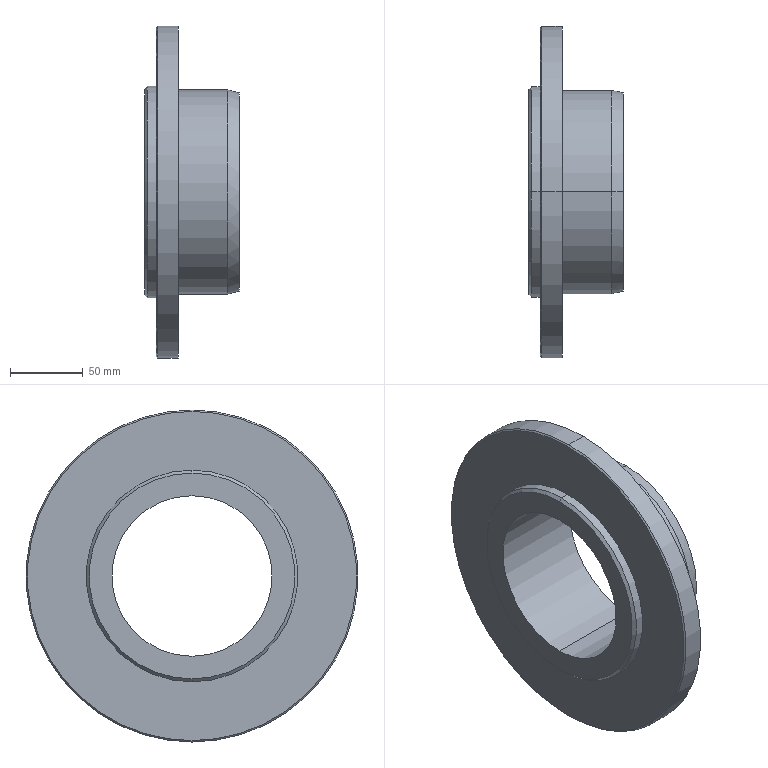Part | STEP file | Labyrinth cover | 1 solid | 27 faces | box 65 x 227.5 x 227.5 mm | volume 634652 mm3 | cylinder 14 | plane 7 | cone 6 | commonest cylinder face diameters 110 x2 140 x2 145 x2 180.5 x2 191.5 x2 218 x2